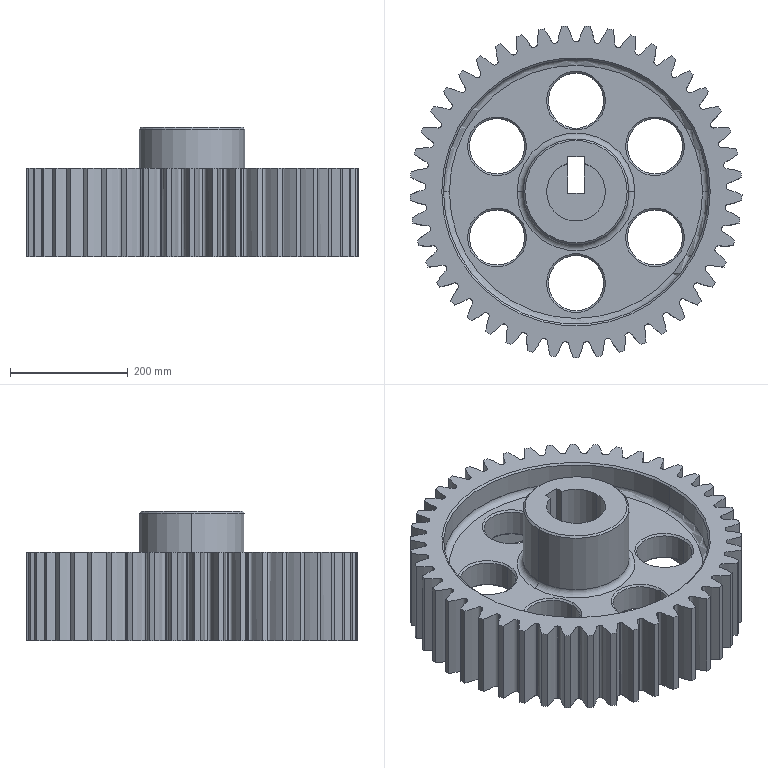Part | SolidWorks | features ICE 8, Chamfer 2, CirPattern 1, Extrusion 1, Fillet 1, RefAxis 1 | 1 solid | 254 faces | box 563.903 x 563.597 x 220 mm | volume 18785882 mm3 | cylinder 113 | spline 90 | cone 32 | plane 11 | torus 8 | commonest cylinder face diameters 510 x45 564 x45 93.872 x12 180 x4 450 x4 100 x3